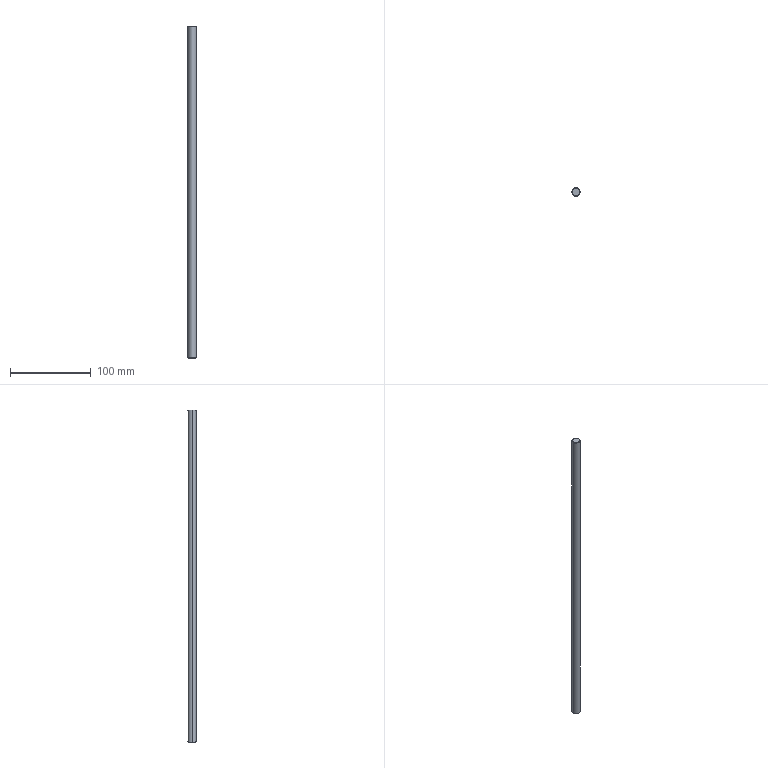Part | STEP file | 1 solid | 8 faces | box 10 x 10 x 411 mm | volume 32272 mm3 | cone 4 | plane 2 | cylinder 2 | commonest cylinder face diameters 10 x2
STEP:
#1=CARTESIAN_POINT('',(0.,0.,0.));
#2=DIRECTION('',(0.,0.,1.));
#3=DIRECTION('',(1.,0.,0.));
#4=AXIS2_PLACEMENT_3D('',#1,#2,#3);
#5=CARTESIAN_POINT('',(-5.,0.,410.5));
#6=VERTEX_POINT('',#5);
#7=CARTESIAN_POINT('',(-4.5,0.,411.));
#8=VERTEX_POINT('',#7);
#9=CARTESIAN_POINT('',(-5.,0.,410.5));
#10=DIRECTION('',(0.7071,0.,0.7071));
#11=VECTOR('',#10,1.);
#12=LINE('',#9,#11);
#13=CARTESIAN_POINT('',(0.,0.,411.025));
#14=DIRECTION('',(0.,0.,-1.));
#15=DIRECTION('',(-1.,0.,0.));
#16=AXIS2_PLACEMENT_3D('',#13,#14,#15);
#17=CONICAL_SURFACE('',#16,4.475,0.7854);
#18=CARTESIAN_POINT('',(0.,0.525));
#19=DIRECTION('',(0.,-1.));
#20=VECTOR('',#19,1.);
#21=LINE('',#18,#20);
#22=(GEOMETRIC_REPRESENTATION_CONTEXT(2)PARAMETRIC_REPRESENTATION_CONTEXT()REPRESENTATION_CONTEXT('',''));
#23=DEFINITIONAL_REPRESENTATION('',(#21),#22);
#24=PCURVE('',#17,#23);
#25=CARTESIAN_POINT('',(0.,0.,411.025));
#26=DIRECTION('',(0.,0.,-1.));
#27=DIRECTION('',(-1.,0.,0.));
#28=AXIS2_PLACEMENT_3D('',#25,#26,#27);
#29=CONICAL_SURFACE('',#28,4.475,0.7854);
#30=CARTESIAN_POINT('',(6.283,0.525));
#31=DIRECTION('',(0.,-1.));
#32=VECTOR('',#31,1.);
#33=LINE('',#30,#32);
#34=(GEOMETRIC_REPRESENTATION_CONTEXT(2)PARAMETRIC_REPRESENTATION_CONTEXT()REPRESENTATION_CONTEXT('',''));
#35=DEFINITIONAL_REPRESENTATION('',(#33),#34);
#36=PCURVE('',#29,#35);
#37=SURFACE_CURVE('',#12,(#24,#36),.PCURVE_S1.);
#38=EDGE_CURVE('',#6,#8,#37,.T.);
#39=ORIENTED_EDGE('',*,*,#38,.T.);
#40=CARTESIAN_POINT('',(4.5,0.,411.));
#41=VERTEX_POINT('',#40);
#42=CARTESIAN_POINT('',(0.,0.,411.));
#43=DIRECTION('',(0.,0.,1.));
#44=DIRECTION('',(1.,0.,0.));
#45=AXIS2_PLACEMENT_3D('',#42,#43,#44);
#46=CIRCLE('',#45,4.5);
#47=CARTESIAN_POINT('',(3.142,0.025));
#48=DIRECTION('',(-1.,0.));
#49=VECTOR('',#48,1.);
#50=LINE('',#47,#49);
#51=(GEOMETRIC_REPRESENTATION_CONTEXT(2)PARAMETRIC_REPRESENTATION_CONTEXT()REPRESENTATION_CONTEXT('',''));
#52=DEFINITIONAL_REPRESENTATION('',(#50),#51);
#53=PCURVE('',#17,#52);
#54=CARTESIAN_POINT('',(-4.95,-4.95,411.));
#55=DIRECTION('',(0.,0.,1.));
#56=DIRECTION('',(1.,0.,0.));
#57=AXIS2_PLACEMENT_3D('',#54,#55,#56);
#58=PLANE('',#57);
#59=CARTESIAN_POINT('',(4.95,4.95));
#60=DIRECTION('',(1.,0.));
#61=AXIS2_PLACEMENT_2D('',#59,#60);
#62=CIRCLE('',#61,4.5);
#63=(GEOMETRIC_REPRESENTATION_CONTEXT(2)PARAMETRIC_REPRESENTATION_CONTEXT()REPRESENTATION_CONTEXT('',''));
#64=DEFINITIONAL_REPRESENTATION('',(#62),#63);
#65=PCURVE('',#58,#64);
#66=SURFACE_CURVE('',#46,(#53,#65),.PCURVE_S1.);
#67=EDGE_CURVE('',#41,#8,#66,.T.);
#68=ORIENTED_EDGE('',*,*,#67,.F.);
#69=CARTESIAN_POINT('',(5.,0.,410.5));
#70=VERTEX_POINT('',#69);
#71=CARTESIAN_POINT('',(5.,0.,410.5));
#72=DIRECTION('',(-0.7071,0.,0.7071));
#73=VECTOR('',#72,1.);
#74=LINE('',#71,#73);
#75=CARTESIAN_POINT('',(3.142,0.525));
#76=DIRECTION('',(0.,-1.));
#77=VECTOR('',#76,1.);
#78=LINE('',#75,#77);
#79=(GEOMETRIC_REPRESENTATION_CONTEXT(2)PARAMETRIC_REPRESENTATION_CONTEXT()REPRESENTATION_CONTEXT('',''));
#80=DEFINITIONAL_REPRESENTATION('',(#78),#79);
#81=PCURVE('',#17,#80);
#82=CARTESIAN_POINT('',(3.142,0.525));
#83=DIRECTION('',(0.,-1.));
#84=VECTOR('',#83,1.);
#85=LINE('',#82,#84);
#86=(GEOMETRIC_REPRESENTATION_CONTEXT(2)PARAMETRIC_REPRESENTATION_CONTEXT()REPRESENTATION_CONTEXT('',''));
#87=DEFINITIONAL_REPRESENTATION('',(#85),#86);
#88=PCURVE('',#29,#87);
#89=SURFACE_CURVE('',#74,(#81,#88),.PCURVE_S1.);
#90=EDGE_CURVE('',#70,#41,#89,.T.);
#91=ORIENTED_EDGE('',*,*,#90,.F.);
#92=CARTESIAN_POINT('',(0.,0.,410.5));
#93=DIRECTION('',(0.,0.,-1.));
#94=DIRECTION('',(1.,0.,0.));
#95=AXIS2_PLACEMENT_3D('',#92,#93,#94);
#96=CIRCLE('',#95,5.);
#97=CARTESIAN_POINT('',(-3.142,0.525));
#98=DIRECTION('',(1.,0.));
#99=VECTOR('',#98,1.);
#100=LINE('',#97,#99);
#101=(GEOMETRIC_REPRESENTATION_CONTEXT(2)PARAMETRIC_REPRESENTATION_CONTEXT()REPRESENTATION_CONTEXT('',''));
#102=DEFINITIONAL_REPRESENTATION('',(#100),#101);
#103=PCURVE('',#17,#102);
#104=CARTESIAN_POINT('',(0.,0.,511.));
#105=DIRECTION('',(0.,0.,-1.));
#106=DIRECTION('',(-1.,0.,0.));
#107=AXIS2_PLACEMENT_3D('',#104,#105,#106);
#108=CYLINDRICAL_SURFACE('',#107,5.);
#109=CARTESIAN_POINT('',(-3.142,100.5));
#110=DIRECTION('',(1.,0.));
#111=VECTOR('',#110,1.);
#112=LINE('',#109,#111);
#113=(GEOMETRIC_REPRESENTATION_CONTEXT(2)PARAMETRIC_REPRESENTATION_CONTEXT()REPRESENTATION_CONTEXT('',''));
#114=DEFINITIONAL_REPRESENTATION('',(#112),#113);
#115=PCURVE('',#108,#114);
#116=SURFACE_CURVE('',#96,(#103,#115),.PCURVE_S1.);
#117=EDGE_CURVE('',#6,#70,#116,.T.);
#118=ORIENTED_EDGE('',*,*,#117,.F.);
#119=EDGE_LOOP('',(#39,#68,#91,#118));
#120=FACE_BOUND('',#119,.T.);
#121=ADVANCED_FACE('',(#120),#17,.T.);
#122=ORIENTED_EDGE('',*,*,#67,.T.);
#123=CARTESIAN_POINT('',(0.,0.,411.));
#124=DIRECTION('',(0.,0.,1.));
#125=DIRECTION('',(1.,0.,0.));
#126=AXIS2_PLACEMENT_3D('',#123,#124,#125);
#127=CIRCLE('',#126,4.5);
#128=CARTESIAN_POINT('',(4.95,4.95));
#129=DIRECTION('',(1.,0.));
#130=AXIS2_PLACEMENT_2D('',#128,#129);
#131=CIRCLE('',#130,4.5);
#132=(GEOMETRIC_REPRESENTATION_CONTEXT(2)PARAMETRIC_REPRESENTATION_CONTEXT()REPRESENTATION_CONTEXT('',''));
#133=DEFINITIONAL_REPRESENTATION('',(#131),#132);
#134=PCURVE('',#58,#133);
#135=CARTESIAN_POINT('',(9.425,0.025));
#136=DIRECTION('',(-1.,0.));
#137=VECTOR('',#136,1.);
#138=LINE('',#135,#137);
#139=(GEOMETRIC_REPRESENTATION_CONTEXT(2)PARAMETRIC_REPRESENTATION_CONTEXT()REPRESENTATION_CONTEXT('',''));
#140=DEFINITIONAL_REPRESENTATION('',(#138),#139);
#141=PCURVE('',#29,#140);
#142=SURFACE_CURVE('',#127,(#134,#141),.PCURVE_S1.);
#143=EDGE_CURVE('',#8,#41,#142,.T.);
#144=ORIENTED_EDGE('',*,*,#143,.T.);
#145=EDGE_LOOP('',(#122,#144));
#146=FACE_BOUND('',#145,.T.);
#147=ADVANCED_FACE('',(#146),#58,.T.);
#148=CARTESIAN_POINT('',(4.5,0.,0.));
#149=VERTEX_POINT('',#148);
#150=CARTESIAN_POINT('',(-4.5,0.,0.));
#151=VERTEX_POINT('',#150);
#152=CARTESIAN_POINT('',(0.,0.,0.));
#153=DIRECTION('',(0.,0.,-1.));
#154=DIRECTION('',(1.,0.,0.));
#155=AXIS2_PLACEMENT_3D('',#152,#153,#154);
#156=CIRCLE('',#155,4.5);
#157=CARTESIAN_POINT('',(-4.95,-4.95,0.));
#158=DIRECTION('',(0.,0.,1.));
#159=DIRECTION('',(1.,0.,0.));
#160=AXIS2_PLACEMENT_3D('',#157,#158,#159);
#161=PLANE('',#160);
#162=CARTESIAN_POINT('',(9.45,4.95));
#163=CARTESIAN_POINT('',(9.45,-2.844));
#164=CARTESIAN_POINT('',(2.7,1.053));
#165=CARTESIAN_POINT('',(-4.05,4.95));
#166=CARTESIAN_POINT('',(2.7,8.847));
#167=CARTESIAN_POINT('',(9.45,12.744));
#168=CARTESIAN_POINT('',(9.45,4.95));
#169=(BOUNDED_CURVE()B_SPLINE_CURVE(2,(#162,#163,#164,#165,#166,#167,#168),.UNSPECIFIED.,.T.,.F.)B_SPLINE_CURVE_WITH_KNOTS((1,2,2,2,2,1),(-2.094,0.,2.094,4.189,6.283,8.378),.UNSPECIFIED.)CURVE()GEOMETRIC_REPRESENTATION_ITEM()RATIONAL_B_SPLINE_CURVE((1.,0.5,1.,0.5,1.,0.5,1.))REPRESENTATION_ITEM(''));
#170=(GEOMETRIC_REPRESENTATION_CONTEXT(2)PARAMETRIC_REPRESENTATION_CONTEXT()REPRESENTATION_CONTEXT('',''));
#171=DEFINITIONAL_REPRESENTATION('',(#169),#170);
#172=PCURVE('',#161,#171);
#173=CARTESIAN_POINT('',(0.,0.,-0.025));
#174=DIRECTION('',(0.,0.,1.));
#175=DIRECTION('',(1.,0.,0.));
#176=AXIS2_PLACEMENT_3D('',#173,#174,#175);
#177=CONICAL_SURFACE('',#176,4.475,0.7854);
#178=CARTESIAN_POINT('',(6.283,0.025));
#179=DIRECTION('',(-1.,0.));
#180=VECTOR('',#179,1.);
#181=LINE('',#178,#180);
#182=(GEOMETRIC_REPRESENTATION_CONTEXT(2)PARAMETRIC_REPRESENTATION_CONTEXT()REPRESENTATION_CONTEXT('',''));
#183=DEFINITIONAL_REPRESENTATION('',(#181),#182);
#184=PCURVE('',#177,#183);
#185=SURFACE_CURVE('',#156,(#172,#184),.PCURVE_S1.);
#186=EDGE_CURVE('',#149,#151,#185,.T.);
#187=ORIENTED_EDGE('',*,*,#186,.T.);
#188=CARTESIAN_POINT('',(0.,0.,0.));
#189=DIRECTION('',(0.,0.,-1.));
#190=DIRECTION('',(1.,0.,0.));
#191=AXIS2_PLACEMENT_3D('',#188,#189,#190);
#192=CIRCLE('',#191,4.5);
#193=CARTESIAN_POINT('',(9.45,4.95));
#194=CARTESIAN_POINT('',(9.45,-2.844));
#195=CARTESIAN_POINT('',(2.7,1.053));
#196=CARTESIAN_POINT('',(-4.05,4.95));
#197=CARTESIAN_POINT('',(2.7,8.847));
#198=CARTESIAN_POINT('',(9.45,12.744));
#199=CARTESIAN_POINT('',(9.45,4.95));
#200=(BOUNDED_CURVE()B_SPLINE_CURVE(2,(#193,#194,#195,#196,#197,#198,#199),.UNSPECIFIED.,.T.,.F.)B_SPLINE_CURVE_WITH_KNOTS((1,2,2,2,2,1),(-2.094,0.,2.094,4.189,6.283,8.378),.UNSPECIFIED.)CURVE()GEOMETRIC_REPRESENTATION_ITEM()RATIONAL_B_SPLINE_CURVE((1.,0.5,1.,0.5,1.,0.5,1.))REPRESENTATION_ITEM(''));
#201=(GEOMETRIC_REPRESENTATION_CONTEXT(2)PARAMETRIC_REPRESENTATION_CONTEXT()REPRESENTATION_CONTEXT('',''));
#202=DEFINITIONAL_REPRESENTATION('',(#200),#201);
#203=PCURVE('',#161,#202);
#204=CARTESIAN_POINT('',(0.,0.,-0.025));
#205=DIRECTION('',(0.,0.,1.));
#206=DIRECTION('',(1.,0.,0.));
#207=AXIS2_PLACEMENT_3D('',#204,#205,#206);
#208=CONICAL_SURFACE('',#207,4.475,0.7854);
#209=CARTESIAN_POINT('',(6.283,0.025));
#210=DIRECTION('',(-1.,0.));
#211=VECTOR('',#210,1.);
#212=LINE('',#209,#211);
#213=(GEOMETRIC_REPRESENTATION_CONTEXT(2)PARAMETRIC_REPRESENTATION_CONTEXT()REPRESENTATION_CONTEXT('',''));
#214=DEFINITIONAL_REPRESENTATION('',(#212),#213);
#215=PCURVE('',#208,#214);
#216=SURFACE_CURVE('',#192,(#203,#215),.PCURVE_S1.);
#217=EDGE_CURVE('',#151,#149,#216,.T.);
#218=ORIENTED_EDGE('',*,*,#217,.T.);
#219=EDGE_LOOP('',(#187,#218));
#220=FACE_BOUND('',#219,.T.);
#221=ADVANCED_FACE('',(#220),#161,.F.);
#222=CARTESIAN_POINT('',(5.,0.,0.5));
#223=VERTEX_POINT('',#222);
#224=CARTESIAN_POINT('',(5.,0.,0.5));
#225=DIRECTION('',(-0.7071,0.,-0.7071));
#226=VECTOR('',#225,1.);
#227=LINE('',#224,#226);
#228=CARTESIAN_POINT('',(0.,0.525));
#229=DIRECTION('',(0.,-1.));
#230=VECTOR('',#229,1.);
#231=LINE('',#228,#230);
#232=(GEOMETRIC_REPRESENTATION_CONTEXT(2)PARAMETRIC_REPRESENTATION_CONTEXT()REPRESENTATION_CONTEXT('',''));
#233=DEFINITIONAL_REPRESENTATION('',(#231),#232);
#234=PCURVE('',#208,#233);
#235=CARTESIAN_POINT('',(6.283,0.525));
#236=DIRECTION('',(0.,-1.));
#237=VECTOR('',#236,1.);
#238=LINE('',#235,#237);
#239=(GEOMETRIC_REPRESENTATION_CONTEXT(2)PARAMETRIC_REPRESENTATION_CONTEXT()REPRESENTATION_CONTEXT('',''));
#240=DEFINITIONAL_REPRESENTATION('',(#238),#239);
#241=PCURVE('',#177,#240);
#242=SURFACE_CURVE('',#227,(#234,#241),.PCURVE_S1.);
#243=EDGE_CURVE('',#223,#149,#242,.T.);
#244=ORIENTED_EDGE('',*,*,#243,.T.);
#245=ORIENTED_EDGE('',*,*,#217,.F.);
#246=CARTESIAN_POINT('',(-5.,0.,0.5));
#247=VERTEX_POINT('',#246);
#248=CARTESIAN_POINT('',(-5.,0.,0.5));
#249=DIRECTION('',(0.7071,0.,-0.7071));
#250=VECTOR('',#249,1.);
#251=LINE('',#248,#250);
#252=CARTESIAN_POINT('',(3.142,0.525));
#253=DIRECTION('',(0.,-1.));
#254=VECTOR('',#253,1.);
#255=LINE('',#252,#254);
#256=(GEOMETRIC_REPRESENTATION_CONTEXT(2)PARAMETRIC_REPRESENTATION_CONTEXT()REPRESENTATION_CONTEXT('',''));
#257=DEFINITIONAL_REPRESENTATION('',(#255),#256);
#258=PCURVE('',#208,#257);
#259=CARTESIAN_POINT('',(3.142,0.525));
#260=DIRECTION('',(0.,-1.));
#261=VECTOR('',#260,1.);
#262=LINE('',#259,#261);
#263=(GEOMETRIC_REPRESENTATION_CONTEXT(2)PARAMETRIC_REPRESENTATION_CONTEXT()REPRESENTATION_CONTEXT('',''));
#264=DEFINITIONAL_REPRESENTATION('',(#262),#263);
#265=PCURVE('',#177,#264);
#266=SURFACE_CURVE('',#251,(#258,#265),.PCURVE_S1.);
#267=EDGE_CURVE('',#247,#151,#266,.T.);
#268=ORIENTED_EDGE('',*,*,#267,.F.);
#269=CARTESIAN_POINT('',(0.,0.,0.5));
#270=DIRECTION('',(0.,0.,1.));
#271=DIRECTION('',(1.,0.,0.));
#272=AXIS2_PLACEMENT_3D('',#269,#270,#271);
#273=CIRCLE('',#272,5.);
#274=CARTESIAN_POINT('',(0.,0.525));
#275=DIRECTION('',(1.,0.));
#276=VECTOR('',#275,1.);
#277=LINE('',#274,#276);
#278=(GEOMETRIC_REPRESENTATION_CONTEXT(2)PARAMETRIC_REPRESENTATION_CONTEXT()REPRESENTATION_CONTEXT('',''));
#279=DEFINITIONAL_REPRESENTATION('',(#277),#278);
#280=PCURVE('',#208,#279);
#281=CARTESIAN_POINT('',(3.142,510.5));
#282=DIRECTION('',(-1.,0.));
#283=VECTOR('',#282,1.);
#284=LINE('',#281,#283);
#285=(GEOMETRIC_REPRESENTATION_CONTEXT(2)PARAMETRIC_REPRESENTATION_CONTEXT()REPRESENTATION_CONTEXT('',''));
#286=DEFINITIONAL_REPRESENTATION('',(#284),#285);
#287=PCURVE('',#108,#286);
#288=SURFACE_CURVE('',#273,(#280,#287),.PCURVE_S1.);
#289=EDGE_CURVE('',#223,#247,#288,.T.);
#290=ORIENTED_EDGE('',*,*,#289,.F.);
#291=EDGE_LOOP('',(#244,#245,#268,#290));
#292=FACE_BOUND('',#291,.T.);
#293=ADVANCED_FACE('',(#292),#208,.T.);
#294=CARTESIAN_POINT('',(-5.,0.,0.5));
#295=DIRECTION('',(0.,0.,1.));
#296=VECTOR('',#295,1.);
#297=LINE('',#294,#296);
#298=CARTESIAN_POINT('',(0.,510.5));
#299=DIRECTION('',(0.,-1.));
#300=VECTOR('',#299,1.);
#301=LINE('',#298,#300);
#302=(GEOMETRIC_REPRESENTATION_CONTEXT(2)PARAMETRIC_REPRESENTATION_CONTEXT()REPRESENTATION_CONTEXT('',''));
#303=DEFINITIONAL_REPRESENTATION('',(#301),#302);
#304=PCURVE('',#108,#303);
#305=CARTESIAN_POINT('',(0.,0.,511.));
#306=DIRECTION('',(0.,0.,-1.));
#307=DIRECTION('',(-1.,0.,0.));
#308=AXIS2_PLACEMENT_3D('',#305,#306,#307);
#309=CYLINDRICAL_SURFACE('',#308,5.);
#310=CARTESIAN_POINT('',(6.283,510.5));
#311=DIRECTION('',(0.,-1.));
#312=VECTOR('',#311,1.);
#313=LINE('',#310,#312);
#314=(GEOMETRIC_REPRESENTATION_CONTEXT(2)PARAMETRIC_REPRESENTATION_CONTEXT()REPRESENTATION_CONTEXT('',''));
#315=DEFINITIONAL_REPRESENTATION('',(#313),#314);
#316=PCURVE('',#309,#315);
#317=SURFACE_CURVE('',#297,(#304,#316),.PCURVE_S1.);
#318=EDGE_CURVE('',#247,#6,#317,.T.);
#319=ORIENTED_EDGE('',*,*,#318,.T.);
#320=ORIENTED_EDGE('',*,*,#117,.T.);
#321=CARTESIAN_POINT('',(5.,0.,0.5));
#322=DIRECTION('',(0.,0.,1.));
#323=VECTOR('',#322,1.);
#324=LINE('',#321,#323);
#325=CARTESIAN_POINT('',(3.142,510.5));
#326=DIRECTION('',(0.,-1.));
#327=VECTOR('',#326,1.);
#328=LINE('',#325,#327);
#329=(GEOMETRIC_REPRESENTATION_CONTEXT(2)PARAMETRIC_REPRESENTATION_CONTEXT()REPRESENTATION_CONTEXT('',''));
#330=DEFINITIONAL_REPRESENTATION('',(#328),#329);
#331=PCURVE('',#108,#330);
#332=CARTESIAN_POINT('',(3.142,510.5));
#333=DIRECTION('',(0.,-1.));
#334=VECTOR('',#333,1.);
#335=LINE('',#332,#334);
#336=(GEOMETRIC_REPRESENTATION_CONTEXT(2)PARAMETRIC_REPRESENTATION_CONTEXT()REPRESENTATION_CONTEXT('',''));
#337=DEFINITIONAL_REPRESENTATION('',(#335),#336);
#338=PCURVE('',#309,#337);
#339=SURFACE_CURVE('',#324,(#331,#338),.PCURVE_S1.);
#340=EDGE_CURVE('',#223,#70,#339,.T.);
#341=ORIENTED_EDGE('',*,*,#340,.F.);
#342=ORIENTED_EDGE('',*,*,#289,.T.);
#343=EDGE_LOOP('',(#319,#320,#341,#342));
#344=FACE_BOUND('',#343,.T.);
#345=ADVANCED_FACE('',(#344),#108,.T.);
#346=ORIENTED_EDGE('',*,*,#318,.F.);
#347=CARTESIAN_POINT('',(0.,0.,0.5));
#348=DIRECTION('',(0.,0.,1.));
#349=DIRECTION('',(1.,0.,0.));
#350=AXIS2_PLACEMENT_3D('',#347,#348,#349);
#351=CIRCLE('',#350,5.);
#352=CARTESIAN_POINT('',(9.425,510.5));
#353=DIRECTION('',(-1.,0.));
#354=VECTOR('',#353,1.);
#355=LINE('',#352,#354);
#356=(GEOMETRIC_REPRESENTATION_CONTEXT(2)PARAMETRIC_REPRESENTATION_CONTEXT()REPRESENTATION_CONTEXT('',''));
#357=DEFINITIONAL_REPRESENTATION('',(#355),#356);
#358=PCURVE('',#309,#357);
#359=CARTESIAN_POINT('',(0.,0.525));
#360=DIRECTION('',(1.,0.));
#361=VECTOR('',#360,1.);
#362=LINE('',#359,#361);
#363=(GEOMETRIC_REPRESENTATION_CONTEXT(2)PARAMETRIC_REPRESENTATION_CONTEXT()REPRESENTATION_CONTEXT('',''));
#364=DEFINITIONAL_REPRESENTATION('',(#362),#363);
#365=PCURVE('',#177,#364);
#366=SURFACE_CURVE('',#351,(#358,#365),.PCURVE_S1.);
#367=EDGE_CURVE('',#247,#223,#366,.T.);
#368=ORIENTED_EDGE('',*,*,#367,.T.);
#369=ORIENTED_EDGE('',*,*,#340,.T.);
#370=CARTESIAN_POINT('',(0.,0.,410.5));
#371=DIRECTION('',(0.,0.,-1.));
#372=DIRECTION('',(1.,0.,0.));
#373=AXIS2_PLACEMENT_3D('',#370,#371,#372);
#374=CIRCLE('',#373,5.);
#375=CARTESIAN_POINT('',(3.142,100.5));
#376=DIRECTION('',(1.,0.));
#377=VECTOR('',#376,1.);
#378=LINE('',#375,#377);
#379=(GEOMETRIC_REPRESENTATION_CONTEXT(2)PARAMETRIC_REPRESENTATION_CONTEXT()REPRESENTATION_CONTEXT('',''));
#380=DEFINITIONAL_REPRESENTATION('',(#378),#379);
#381=PCURVE('',#309,#380);
#382=CARTESIAN_POINT('',(3.142,0.525));
#383=DIRECTION('',(1.,0.));
#384=VECTOR('',#383,1.);
#385=LINE('',#382,#384);
#386=(GEOMETRIC_REPRESENTATION_CONTEXT(2)PARAMETRIC_REPRESENTATION_CONTEXT()REPRESENTATION_CONTEXT('',''));
#387=DEFINITIONAL_REPRESENTATION('',(#385),#386);
#388=PCURVE('',#29,#387);
#389=SURFACE_CURVE('',#374,(#381,#388),.PCURVE_S1.);
#390=EDGE_CURVE('',#70,#6,#389,.T.);
#391=ORIENTED_EDGE('',*,*,#390,.T.);
#392=EDGE_LOOP('',(#346,#368,#369,#391));
#393=FACE_BOUND('',#392,.T.);
#394=ADVANCED_FACE('',(#393),#309,.T.);
#395=ORIENTED_EDGE('',*,*,#243,.F.);
#396=ORIENTED_EDGE('',*,*,#367,.F.);
#397=ORIENTED_EDGE('',*,*,#267,.T.);
#398=ORIENTED_EDGE('',*,*,#186,.F.);
#399=EDGE_LOOP('',(#395,#396,#397,#398));
#400=FACE_BOUND('',#399,.T.);
#401=ADVANCED_FACE('',(#400),#177,.T.);
#402=ORIENTED_EDGE('',*,*,#38,.F.);
#403=ORIENTED_EDGE('',*,*,#390,.F.);
#404=ORIENTED_EDGE('',*,*,#90,.T.);
#405=ORIENTED_EDGE('',*,*,#143,.F.);
#406=EDGE_LOOP('',(#402,#403,#404,#405));
#407=FACE_BOUND('',#406,.T.);
#408=ADVANCED_FACE('',(#407),#29,.T.);
#409=CLOSED_SHELL('',(#121,#147,#221,#293,#345,#394,#401,#408));
#410=MANIFOLD_SOLID_BREP('',#409);
#411=(LENGTH_UNIT()NAMED_UNIT(*)SI_UNIT(.MILLI.,.METRE.));
#412=UNCERTAINTY_MEASURE_WITH_UNIT(LENGTH_MEASURE(0.0000001),#411,'','');
#413=(NAMED_UNIT(*)PLANE_ANGLE_UNIT()SI_UNIT($,.RADIAN.));
#414=(NAMED_UNIT(*)SI_UNIT($,.STERADIAN.)SOLID_ANGLE_UNIT());
#415=(GEOMETRIC_REPRESENTATION_CONTEXT(3)GLOBAL_UNCERTAINTY_ASSIGNED_CONTEXT((#412))GLOBAL_UNIT_ASSIGNED_CONTEXT((#411,#413,#414))REPRESENTATION_CONTEXT('',''));
#416=ADVANCED_BREP_SHAPE_REPRESENTATION('',(#4,#410),#415);